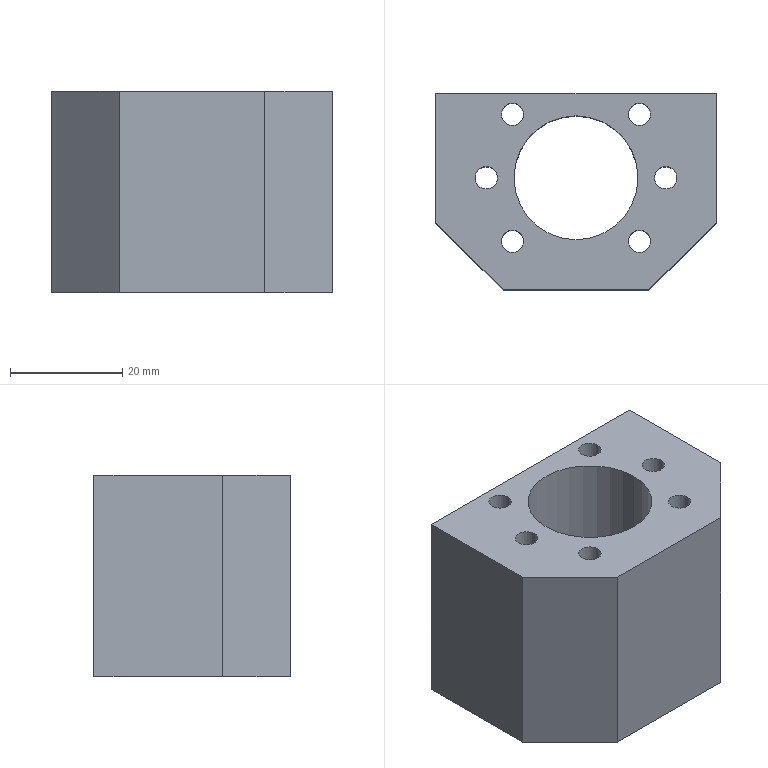Part | SolidWorks | features BaseBody 1 | 1 solid | 34 faces | box 50 x 35 x 36 mm | volume 40507 mm3 | cylinder 22 | plane 12 | commonest cylinder face diameters 4 x12 5 x8 22.1 x2
STEP:
#1=CARTESIAN_POINT('',(-15.,5.,6.));
#2=VERTEX_POINT('',#1);
#3=CARTESIAN_POINT('',(-20.,5.,6.));
#4=VERTEX_POINT('',#3);
#5=CARTESIAN_POINT('',(-17.5,5.,6.));
#6=DIRECTION('',(0.,1.,0.));
#7=DIRECTION('',(-1.,0.,0.));
#8=AXIS2_PLACEMENT_3D('',#5,#6,#7);
#9=CIRCLE('',#8,2.5);
#10=EDGE_CURVE('',#2,#4,#9,.T.);
#11=ORIENTED_EDGE('',*,*,#10,.F.);
#12=CARTESIAN_POINT('',(-15.,15.,6.));
#13=VERTEX_POINT('',#12);
#14=CARTESIAN_POINT('',(-15.,5.,6.));
#15=DIRECTION('',(0.,1.,0.));
#16=VECTOR('',#15,1000.);
#17=LINE('',#14,#16);
#18=EDGE_CURVE('',#2,#13,#17,.T.);
#19=ORIENTED_EDGE('',*,*,#18,.T.);
#20=CARTESIAN_POINT('',(-20.,15.,6.));
#21=VERTEX_POINT('',#20);
#22=CARTESIAN_POINT('',(-17.5,15.,6.));
#23=DIRECTION('',(0.,1.,0.));
#24=DIRECTION('',(-1.,0.,0.));
#25=AXIS2_PLACEMENT_3D('',#22,#23,#24);
#26=CIRCLE('',#25,2.5);
#27=EDGE_CURVE('',#13,#21,#26,.T.);
#28=ORIENTED_EDGE('',*,*,#27,.T.);
#29=CARTESIAN_POINT('',(-20.,5.,6.));
#30=DIRECTION('',(0.,1.,0.));
#31=VECTOR('',#30,1000.);
#32=LINE('',#29,#31);
#33=EDGE_CURVE('',#4,#21,#32,.T.);
#34=ORIENTED_EDGE('',*,*,#33,.F.);
#35=EDGE_LOOP('',(#11,#19,#28,#34));
#36=FACE_OUTER_BOUND('',#35,.T.);
#37=CARTESIAN_POINT('',(-17.5,5.,6.));
#38=DIRECTION('',(0.,1.,0.));
#39=DIRECTION('',(-1.,0.,0.));
#40=AXIS2_PLACEMENT_3D('',#37,#38,#39);
#41=CYLINDRICAL_SURFACE('',#40,2.5);
#42=ADVANCED_FACE('',(#36),#41,.F.);
#43=CARTESIAN_POINT('',(-15.,5.,30.));
#44=VERTEX_POINT('',#43);
#45=CARTESIAN_POINT('',(-20.,5.,30.));
#46=VERTEX_POINT('',#45);
#47=CARTESIAN_POINT('',(-17.5,5.,30.));
#48=DIRECTION('',(0.,1.,0.));
#49=DIRECTION('',(-1.,0.,0.));
#50=AXIS2_PLACEMENT_3D('',#47,#48,#49);
#51=CIRCLE('',#50,2.5);
#52=EDGE_CURVE('',#44,#46,#51,.T.);
#53=ORIENTED_EDGE('',*,*,#52,.F.);
#54=CARTESIAN_POINT('',(-15.,15.,30.));
#55=VERTEX_POINT('',#54);
#56=CARTESIAN_POINT('',(-15.,5.,30.));
#57=DIRECTION('',(0.,1.,0.));
#58=VECTOR('',#57,1000.);
#59=LINE('',#56,#58);
#60=EDGE_CURVE('',#44,#55,#59,.T.);
#61=ORIENTED_EDGE('',*,*,#60,.T.);
#62=CARTESIAN_POINT('',(-20.,15.,30.));
#63=VERTEX_POINT('',#62);
#64=CARTESIAN_POINT('',(-17.5,15.,30.));
#65=DIRECTION('',(0.,1.,0.));
#66=DIRECTION('',(-1.,0.,0.));
#67=AXIS2_PLACEMENT_3D('',#64,#65,#66);
#68=CIRCLE('',#67,2.5);
#69=EDGE_CURVE('',#55,#63,#68,.T.);
#70=ORIENTED_EDGE('',*,*,#69,.T.);
#71=CARTESIAN_POINT('',(-20.,5.,30.));
#72=DIRECTION('',(0.,1.,0.));
#73=VECTOR('',#72,1000.);
#74=LINE('',#71,#73);
#75=EDGE_CURVE('',#46,#63,#74,.T.);
#76=ORIENTED_EDGE('',*,*,#75,.F.);
#77=EDGE_LOOP('',(#53,#61,#70,#76));
#78=FACE_OUTER_BOUND('',#77,.T.);
#79=CARTESIAN_POINT('',(-17.5,5.,30.));
#80=DIRECTION('',(0.,1.,0.));
#81=DIRECTION('',(-1.,0.,0.));
#82=AXIS2_PLACEMENT_3D('',#79,#80,#81);
#83=CYLINDRICAL_SURFACE('',#82,2.5);
#84=ADVANCED_FACE('',(#78),#83,.F.);
#85=CARTESIAN_POINT('',(20.,5.,30.));
#86=VERTEX_POINT('',#85);
#87=CARTESIAN_POINT('',(15.,5.,30.));
#88=VERTEX_POINT('',#87);
#89=CARTESIAN_POINT('',(17.5,5.,30.));
#90=DIRECTION('',(0.,1.,0.));
#91=DIRECTION('',(-1.,0.,0.));
#92=AXIS2_PLACEMENT_3D('',#89,#90,#91);
#93=CIRCLE('',#92,2.5);
#94=EDGE_CURVE('',#86,#88,#93,.T.);
#95=ORIENTED_EDGE('',*,*,#94,.F.);
#96=CARTESIAN_POINT('',(20.,15.,30.));
#97=VERTEX_POINT('',#96);
#98=CARTESIAN_POINT('',(20.,5.,30.));
#99=DIRECTION('',(0.,1.,0.));
#100=VECTOR('',#99,1000.);
#101=LINE('',#98,#100);
#102=EDGE_CURVE('',#86,#97,#101,.T.);
#103=ORIENTED_EDGE('',*,*,#102,.T.);
#104=CARTESIAN_POINT('',(15.,15.,30.));
#105=VERTEX_POINT('',#104);
#106=CARTESIAN_POINT('',(17.5,15.,30.));
#107=DIRECTION('',(0.,1.,0.));
#108=DIRECTION('',(-1.,0.,0.));
#109=AXIS2_PLACEMENT_3D('',#106,#107,#108);
#110=CIRCLE('',#109,2.5);
#111=EDGE_CURVE('',#97,#105,#110,.T.);
#112=ORIENTED_EDGE('',*,*,#111,.T.);
#113=CARTESIAN_POINT('',(15.,5.,30.));
#114=DIRECTION('',(0.,1.,0.));
#115=VECTOR('',#114,1000.);
#116=LINE('',#113,#115);
#117=EDGE_CURVE('',#88,#105,#116,.T.);
#118=ORIENTED_EDGE('',*,*,#117,.F.);
#119=EDGE_LOOP('',(#95,#103,#112,#118));
#120=FACE_OUTER_BOUND('',#119,.T.);
#121=CARTESIAN_POINT('',(17.5,5.,30.));
#122=DIRECTION('',(0.,1.,0.));
#123=DIRECTION('',(-1.,0.,0.));
#124=AXIS2_PLACEMENT_3D('',#121,#122,#123);
#125=CYLINDRICAL_SURFACE('',#124,2.5);
#126=ADVANCED_FACE('',(#120),#125,.F.);
#127=CARTESIAN_POINT('',(20.,5.,6.));
#128=VERTEX_POINT('',#127);
#129=CARTESIAN_POINT('',(15.,5.,6.));
#130=VERTEX_POINT('',#129);
#131=CARTESIAN_POINT('',(17.5,5.,6.));
#132=DIRECTION('',(0.,1.,0.));
#133=DIRECTION('',(-1.,0.,0.));
#134=AXIS2_PLACEMENT_3D('',#131,#132,#133);
#135=CIRCLE('',#134,2.5);
#136=EDGE_CURVE('',#128,#130,#135,.T.);
#137=ORIENTED_EDGE('',*,*,#136,.F.);
#138=CARTESIAN_POINT('',(20.,15.,6.));
#139=VERTEX_POINT('',#138);
#140=CARTESIAN_POINT('',(20.,5.,6.));
#141=DIRECTION('',(0.,1.,0.));
#142=VECTOR('',#141,1000.);
#143=LINE('',#140,#142);
#144=EDGE_CURVE('',#128,#139,#143,.T.);
#145=ORIENTED_EDGE('',*,*,#144,.T.);
#146=CARTESIAN_POINT('',(15.,15.,6.));
#147=VERTEX_POINT('',#146);
#148=CARTESIAN_POINT('',(17.5,15.,6.));
#149=DIRECTION('',(0.,1.,0.));
#150=DIRECTION('',(-1.,0.,0.));
#151=AXIS2_PLACEMENT_3D('',#148,#149,#150);
#152=CIRCLE('',#151,2.5);
#153=EDGE_CURVE('',#139,#147,#152,.T.);
#154=ORIENTED_EDGE('',*,*,#153,.T.);
#155=CARTESIAN_POINT('',(15.,5.,6.));
#156=DIRECTION('',(0.,1.,0.));
#157=VECTOR('',#156,1000.);
#158=LINE('',#155,#157);
#159=EDGE_CURVE('',#130,#147,#158,.T.);
#160=ORIENTED_EDGE('',*,*,#159,.F.);
#161=EDGE_LOOP('',(#137,#145,#154,#160));
#162=FACE_OUTER_BOUND('',#161,.T.);
#163=CARTESIAN_POINT('',(17.5,5.,6.));
#164=DIRECTION('',(0.,1.,0.));
#165=DIRECTION('',(-1.,0.,0.));
#166=AXIS2_PLACEMENT_3D('',#163,#164,#165);
#167=CYLINDRICAL_SURFACE('',#166,2.5);
#168=ADVANCED_FACE('',(#162),#167,.F.);
#169=CARTESIAN_POINT('',(18.,0.,36.));
#170=VERTEX_POINT('',#169);
#171=CARTESIAN_POINT('',(14.,0.,36.));
#172=VERTEX_POINT('',#171);
#173=CARTESIAN_POINT('',(16.,0.,36.));
#174=DIRECTION('',(0.,0.,-1.));
#175=DIRECTION('',(-1.,0.,0.));
#176=AXIS2_PLACEMENT_3D('',#173,#174,#175);
#177=CIRCLE('',#176,2.);
#178=EDGE_CURVE('',#170,#172,#177,.T.);
#179=ORIENTED_EDGE('',*,*,#178,.F.);
#180=CARTESIAN_POINT('',(18.,0.,0.));
#181=VERTEX_POINT('',#180);
#182=CARTESIAN_POINT('',(18.,0.,36.));
#183=DIRECTION('',(0.,0.,-1.));
#184=VECTOR('',#183,1000.);
#185=LINE('',#182,#184);
#186=EDGE_CURVE('',#170,#181,#185,.T.);
#187=ORIENTED_EDGE('',*,*,#186,.T.);
#188=CARTESIAN_POINT('',(14.,0.,0.));
#189=VERTEX_POINT('',#188);
#190=CARTESIAN_POINT('',(16.,0.,0.));
#191=DIRECTION('',(0.,0.,-1.));
#192=DIRECTION('',(-1.,0.,0.));
#193=AXIS2_PLACEMENT_3D('',#190,#191,#192);
#194=CIRCLE('',#193,2.);
#195=EDGE_CURVE('',#181,#189,#194,.T.);
#196=ORIENTED_EDGE('',*,*,#195,.T.);
#197=CARTESIAN_POINT('',(14.,0.,36.));
#198=DIRECTION('',(0.,0.,-1.));
#199=VECTOR('',#198,1000.);
#200=LINE('',#197,#199);
#201=EDGE_CURVE('',#172,#189,#200,.T.);
#202=ORIENTED_EDGE('',*,*,#201,.F.);
#203=EDGE_LOOP('',(#179,#187,#196,#202));
#204=FACE_OUTER_BOUND('',#203,.T.);
#205=CARTESIAN_POINT('',(16.,0.,36.));
#206=DIRECTION('',(0.,0.,-1.));
#207=DIRECTION('',(-1.,0.,0.));
#208=AXIS2_PLACEMENT_3D('',#205,#206,#207);
#209=CYLINDRICAL_SURFACE('',#208,2.);
#210=ADVANCED_FACE('',(#204),#209,.F.);
#211=CARTESIAN_POINT('',(13.314,11.314,36.));
#212=VERTEX_POINT('',#211);
#213=CARTESIAN_POINT('',(9.314,11.314,36.));
#214=VERTEX_POINT('',#213);
#215=CARTESIAN_POINT('',(11.314,11.314,36.));
#216=DIRECTION('',(0.,0.,-1.));
#217=DIRECTION('',(-1.,0.,0.));
#218=AXIS2_PLACEMENT_3D('',#215,#216,#217);
#219=CIRCLE('',#218,2.);
#220=EDGE_CURVE('',#212,#214,#219,.T.);
#221=ORIENTED_EDGE('',*,*,#220,.F.);
#222=CARTESIAN_POINT('',(13.314,11.314,0.));
#223=VERTEX_POINT('',#222);
#224=CARTESIAN_POINT('',(13.314,11.314,36.));
#225=DIRECTION('',(0.,0.,-1.));
#226=VECTOR('',#225,1000.);
#227=LINE('',#224,#226);
#228=EDGE_CURVE('',#212,#223,#227,.T.);
#229=ORIENTED_EDGE('',*,*,#228,.T.);
#230=CARTESIAN_POINT('',(9.314,11.314,0.));
#231=VERTEX_POINT('',#230);
#232=CARTESIAN_POINT('',(11.314,11.314,0.));
#233=DIRECTION('',(0.,0.,-1.));
#234=DIRECTION('',(-1.,0.,0.));
#235=AXIS2_PLACEMENT_3D('',#232,#233,#234);
#236=CIRCLE('',#235,2.);
#237=EDGE_CURVE('',#223,#231,#236,.T.);
#238=ORIENTED_EDGE('',*,*,#237,.T.);
#239=CARTESIAN_POINT('',(9.314,11.314,36.));
#240=DIRECTION('',(0.,0.,-1.));
#241=VECTOR('',#240,1000.);
#242=LINE('',#239,#241);
#243=EDGE_CURVE('',#214,#231,#242,.T.);
#244=ORIENTED_EDGE('',*,*,#243,.F.);
#245=EDGE_LOOP('',(#221,#229,#238,#244));
#246=FACE_OUTER_BOUND('',#245,.T.);
#247=CARTESIAN_POINT('',(11.314,11.314,36.));
#248=DIRECTION('',(0.,0.,-1.));
#249=DIRECTION('',(-1.,0.,0.));
#250=AXIS2_PLACEMENT_3D('',#247,#248,#249);
#251=CYLINDRICAL_SURFACE('',#250,2.);
#252=ADVANCED_FACE('',(#246),#251,.F.);
#253=CARTESIAN_POINT('',(13.314,-11.314,36.));
#254=VERTEX_POINT('',#253);
#255=CARTESIAN_POINT('',(9.314,-11.314,36.));
#256=VERTEX_POINT('',#255);
#257=CARTESIAN_POINT('',(11.314,-11.314,36.));
#258=DIRECTION('',(0.,0.,-1.));
#259=DIRECTION('',(-1.,0.,0.));
#260=AXIS2_PLACEMENT_3D('',#257,#258,#259);
#261=CIRCLE('',#260,2.);
#262=EDGE_CURVE('',#254,#256,#261,.T.);
#263=ORIENTED_EDGE('',*,*,#262,.F.);
#264=CARTESIAN_POINT('',(13.314,-11.314,0.));
#265=VERTEX_POINT('',#264);
#266=CARTESIAN_POINT('',(13.314,-11.314,36.));
#267=DIRECTION('',(0.,0.,-1.));
#268=VECTOR('',#267,1000.);
#269=LINE('',#266,#268);
#270=EDGE_CURVE('',#254,#265,#269,.T.);
#271=ORIENTED_EDGE('',*,*,#270,.T.);
#272=CARTESIAN_POINT('',(9.314,-11.314,0.));
#273=VERTEX_POINT('',#272);
#274=CARTESIAN_POINT('',(11.314,-11.314,0.));
#275=DIRECTION('',(0.,0.,-1.));
#276=DIRECTION('',(-1.,0.,0.));
#277=AXIS2_PLACEMENT_3D('',#274,#275,#276);
#278=CIRCLE('',#277,2.);
#279=EDGE_CURVE('',#265,#273,#278,.T.);
#280=ORIENTED_EDGE('',*,*,#279,.T.);
#281=CARTESIAN_POINT('',(9.314,-11.314,36.));
#282=DIRECTION('',(0.,0.,-1.));
#283=VECTOR('',#282,1000.);
#284=LINE('',#281,#283);
#285=EDGE_CURVE('',#256,#273,#284,.T.);
#286=ORIENTED_EDGE('',*,*,#285,.F.);
#287=EDGE_LOOP('',(#263,#271,#280,#286));
#288=FACE_OUTER_BOUND('',#287,.T.);
#289=CARTESIAN_POINT('',(11.314,-11.314,36.));
#290=DIRECTION('',(0.,0.,-1.));
#291=DIRECTION('',(-1.,0.,0.));
#292=AXIS2_PLACEMENT_3D('',#289,#290,#291);
#293=CYLINDRICAL_SURFACE('',#292,2.);
#294=ADVANCED_FACE('',(#288),#293,.F.);
#295=CARTESIAN_POINT('',(-9.314,-11.314,36.));
#296=VERTEX_POINT('',#295);
#297=CARTESIAN_POINT('',(-13.314,-11.314,36.));
#298=VERTEX_POINT('',#297);
#299=CARTESIAN_POINT('',(-11.314,-11.314,36.));
#300=DIRECTION('',(0.,0.,-1.));
#301=DIRECTION('',(-1.,0.,0.));
#302=AXIS2_PLACEMENT_3D('',#299,#300,#301);
#303=CIRCLE('',#302,2.);
#304=EDGE_CURVE('',#296,#298,#303,.T.);
#305=ORIENTED_EDGE('',*,*,#304,.F.);
#306=CARTESIAN_POINT('',(-9.314,-11.314,0.));
#307=VERTEX_POINT('',#306);
#308=CARTESIAN_POINT('',(-9.314,-11.314,36.));
#309=DIRECTION('',(0.,0.,-1.));
#310=VECTOR('',#309,1000.);
#311=LINE('',#308,#310);
#312=EDGE_CURVE('',#296,#307,#311,.T.);
#313=ORIENTED_EDGE('',*,*,#312,.T.);
#314=CARTESIAN_POINT('',(-13.314,-11.314,0.));
#315=VERTEX_POINT('',#314);
#316=CARTESIAN_POINT('',(-11.314,-11.314,0.));
#317=DIRECTION('',(0.,0.,-1.));
#318=DIRECTION('',(-1.,0.,0.));
#319=AXIS2_PLACEMENT_3D('',#316,#317,#318);
#320=CIRCLE('',#319,2.);
#321=EDGE_CURVE('',#307,#315,#320,.T.);
#322=ORIENTED_EDGE('',*,*,#321,.T.);
#323=CARTESIAN_POINT('',(-13.314,-11.314,36.));
#324=DIRECTION('',(0.,0.,-1.));
#325=VECTOR('',#324,1000.);
#326=LINE('',#323,#325);
#327=EDGE_CURVE('',#298,#315,#326,.T.);
#328=ORIENTED_EDGE('',*,*,#327,.F.);
#329=EDGE_LOOP('',(#305,#313,#322,#328));
#330=FACE_OUTER_BOUND('',#329,.T.);
#331=CARTESIAN_POINT('',(-11.314,-11.314,36.));
#332=DIRECTION('',(0.,0.,-1.));
#333=DIRECTION('',(-1.,0.,0.));
#334=AXIS2_PLACEMENT_3D('',#331,#332,#333);
#335=CYLINDRICAL_SURFACE('',#334,2.);
#336=ADVANCED_FACE('',(#330),#335,.F.);
#337=CARTESIAN_POINT('',(-9.314,11.314,36.));
#338=VERTEX_POINT('',#337);
#339=CARTESIAN_POINT('',(-13.314,11.314,36.));
#340=VERTEX_POINT('',#339);
#341=CARTESIAN_POINT('',(-11.314,11.314,36.));
#342=DIRECTION('',(0.,0.,-1.));
#343=DIRECTION('',(-1.,0.,0.));
#344=AXIS2_PLACEMENT_3D('',#341,#342,#343);
#345=CIRCLE('',#344,2.);
#346=EDGE_CURVE('',#338,#340,#345,.T.);
#347=ORIENTED_EDGE('',*,*,#346,.F.);
#348=CARTESIAN_POINT('',(-9.314,11.314,0.));
#349=VERTEX_POINT('',#348);
#350=CARTESIAN_POINT('',(-9.314,11.314,36.));
#351=DIRECTION('',(0.,0.,-1.));
#352=VECTOR('',#351,1000.);
#353=LINE('',#350,#352);
#354=EDGE_CURVE('',#338,#349,#353,.T.);
#355=ORIENTED_EDGE('',*,*,#354,.T.);
#356=CARTESIAN_POINT('',(-13.314,11.314,0.));
#357=VERTEX_POINT('',#356);
#358=CARTESIAN_POINT('',(-11.314,11.314,0.));
#359=DIRECTION('',(0.,0.,-1.));
#360=DIRECTION('',(-1.,0.,0.));
#361=AXIS2_PLACEMENT_3D('',#358,#359,#360);
#362=CIRCLE('',#361,2.);
#363=EDGE_CURVE('',#349,#357,#362,.T.);
#364=ORIENTED_EDGE('',*,*,#363,.T.);
#365=CARTESIAN_POINT('',(-13.314,11.314,36.));
#366=DIRECTION('',(0.,0.,-1.));
#367=VECTOR('',#366,1000.);
#368=LINE('',#365,#367);
#369=EDGE_CURVE('',#340,#357,#368,.T.);
#370=ORIENTED_EDGE('',*,*,#369,.F.);
#371=EDGE_LOOP('',(#347,#355,#364,#370));
#372=FACE_OUTER_BOUND('',#371,.T.);
#373=CARTESIAN_POINT('',(-11.314,11.314,36.));
#374=DIRECTION('',(0.,0.,-1.));
#375=DIRECTION('',(-1.,0.,0.));
#376=AXIS2_PLACEMENT_3D('',#373,#374,#375);
#377=CYLINDRICAL_SURFACE('',#376,2.);
#378=ADVANCED_FACE('',(#372),#377,.F.);
#379=CARTESIAN_POINT('',(-14.,0.,36.));
#380=VERTEX_POINT('',#379);
#381=CARTESIAN_POINT('',(-18.,0.,36.));
#382=VERTEX_POINT('',#381);
#383=CARTESIAN_POINT('',(-16.,0.,36.));
#384=DIRECTION('',(0.,0.,-1.));
#385=DIRECTION('',(-1.,0.,0.));
#386=AXIS2_PLACEMENT_3D('',#383,#384,#385);
#387=CIRCLE('',#386,2.);
#388=EDGE_CURVE('',#380,#382,#387,.T.);
#389=ORIENTED_EDGE('',*,*,#388,.F.);
#390=CARTESIAN_POINT('',(-14.,0.,0.));
#391=VERTEX_POINT('',#390);
#392=CARTESIAN_POINT('',(-14.,0.,36.));
#393=DIRECTION('',(0.,0.,-1.));
#394=VECTOR('',#393,1000.);
#395=LINE('',#392,#394);
#396=EDGE_CURVE('',#380,#391,#395,.T.);
#397=ORIENTED_EDGE('',*,*,#396,.T.);
#398=CARTESIAN_POINT('',(-18.,0.,0.));
#399=VERTEX_POINT('',#398);
#400=CARTESIAN_POINT('',(-16.,0.,0.));
#401=DIRECTION('',(0.,0.,-1.));
#402=DIRECTION('',(-1.,0.,0.));
#403=AXIS2_PLACEMENT_3D('',#400,#401,#402);
#404=CIRCLE('',#403,2.);
#405=EDGE_CURVE('',#391,#399,#404,.T.);
#406=ORIENTED_EDGE('',*,*,#405,.T.);
#407=CARTESIAN_POINT('',(-18.,0.,36.));
#408=DIRECTION('',(0.,0.,-1.));
#409=VECTOR('',#408,1000.);
#410=LINE('',#407,#409);
#411=EDGE_CURVE('',#382,#399,#410,.T.);
#412=ORIENTED_EDGE('',*,*,#411,.F.);
#413=EDGE_LOOP('',(#389,#397,#406,#412));
#414=FACE_OUTER_BOUND('',#413,.T.);
#415=CARTESIAN_POINT('',(-16.,0.,36.));
#416=DIRECTION('',(0.,0.,-1.));
#417=DIRECTION('',(-1.,0.,0.));
#418=AXIS2_PLACEMENT_3D('',#415,#416,#417);
#419=CYLINDRICAL_SURFACE('',#418,2.);
#420=ADVANCED_FACE('',(#414),#419,.F.);
#421=CARTESIAN_POINT('',(11.05,0.,36.));
#422=VERTEX_POINT('',#421);
#423=CARTESIAN_POINT('',(-11.05,0.,36.));
#424=VERTEX_POINT('',#423);
#425=CARTESIAN_POINT('',(0.,0.,36.));
#426=DIRECTION('',(0.,0.,-1.));
#427=DIRECTION('',(-1.,0.,0.));
#428=AXIS2_PLACEMENT_3D('',#425,#426,#427);
#429=CIRCLE('',#428,11.05);
#430=EDGE_CURVE('',#422,#424,#429,.T.);
#431=ORIENTED_EDGE('',*,*,#430,.F.);
#432=CARTESIAN_POINT('',(11.05,0.,0.));
#433=VERTEX_POINT('',#432);
#434=CARTESIAN_POINT('',(11.05,0.,36.));
#435=DIRECTION('',(0.,0.,-1.));
#436=VECTOR('',#435,1000.);
#437=LINE('',#434,#436);
#438=EDGE_CURVE('',#422,#433,#437,.T.);
#439=ORIENTED_EDGE('',*,*,#438,.T.);
#440=CARTESIAN_POINT('',(-11.05,0.,0.));
#441=VERTEX_POINT('',#440);
#442=CARTESIAN_POINT('',(0.,0.,0.));
#443=DIRECTION('',(0.,0.,-1.));
#444=DIRECTION('',(-1.,0.,0.));
#445=AXIS2_PLACEMENT_3D('',#442,#443,#444);
#446=CIRCLE('',#445,11.05);
#447=EDGE_CURVE('',#433,#441,#446,.T.);
#448=ORIENTED_EDGE('',*,*,#447,.T.);
#449=CARTESIAN_POINT('',(-11.05,0.,36.));
#450=DIRECTION('',(0.,0.,-1.));
#451=VECTOR('',#450,1000.);
#452=LINE('',#449,#451);
#453=EDGE_CURVE('',#424,#441,#452,.T.);
#454=ORIENTED_EDGE('',*,*,#453,.F.);
#455=EDGE_LOOP('',(#431,#439,#448,#454));
#456=FACE_OUTER_BOUND('',#455,.T.);
#457=CARTESIAN_POINT('',(0.,0.,36.));
#458=DIRECTION('',(0.,0.,-1.));
#459=DIRECTION('',(-1.,0.,0.));
#460=AXIS2_PLACEMENT_3D('',#457,#458,#459);
#461=CYLINDRICAL_SURFACE('',#460,11.05);
#462=ADVANCED_FACE('',(#456),#461,.F.);
#463=CARTESIAN_POINT('',(-25.,15.,36.));
#464=VERTEX_POINT('',#463);
#465=CARTESIAN_POINT('',(-25.,15.,0.));
#466=VERTEX_POINT('',#465);
#467=CARTESIAN_POINT('',(-25.,15.,36.));
#468=DIRECTION('',(0.,0.,-1.));
#469=VECTOR('',#468,1000.);
#470=LINE('',#467,#469);
#471=EDGE_CURVE('',#464,#466,#470,.T.);
#472=ORIENTED_EDGE('',*,*,#471,.F.);
#473=CARTESIAN_POINT('',(25.,15.,36.));
#474=VERTEX_POINT('',#473);
#475=CARTESIAN_POINT('',(25.,15.,36.));
#476=DIRECTION('',(-1.,0.,0.));
#477=VECTOR('',#476,1000.);
#478=LINE('',#475,#477);
#479=EDGE_CURVE('',#474,#464,#478,.T.);
#480=ORIENTED_EDGE('',*,*,#479,.F.);
#481=CARTESIAN_POINT('',(25.,15.,0.));
#482=VERTEX_POINT('',#481);
#483=CARTESIAN_POINT('',(25.,15.,36.));
#484=DIRECTION('',(0.,0.,1.));
#485=VECTOR('',#484,1000.);
#486=LINE('',#483,#485);
#487=EDGE_CURVE('',#482,#474,#486,.T.);
#488=ORIENTED_EDGE('',*,*,#487,.F.);
#489=CARTESIAN_POINT('',(25.,15.,0.));
#490=DIRECTION('',(1.,0.,0.));
#491=VECTOR('',#490,1000.);
#492=LINE('',#489,#491);
#493=EDGE_CURVE('',#466,#482,#492,.T.);
#494=ORIENTED_EDGE('',*,*,#493,.F.);
#495=EDGE_LOOP('',(#472,#480,#488,#494));
#496=FACE_OUTER_BOUND('',#495,.T.);
#497=CARTESIAN_POINT('',(-17.5,15.,6.));
#498=DIRECTION('',(0.,1.,0.));
#499=DIRECTION('',(-1.,0.,0.));
#500=AXIS2_PLACEMENT_3D('',#497,#498,#499);
#501=CIRCLE('',#500,2.5);
#502=EDGE_CURVE('',#21,#13,#501,.T.);
#503=ORIENTED_EDGE('',*,*,#502,.F.);
#504=ORIENTED_EDGE('',*,*,#27,.F.);
#505=EDGE_LOOP('',(#503,#504));
#506=FACE_BOUND('',#505,.T.);
#507=CARTESIAN_POINT('',(-17.5,15.,30.));
#508=DIRECTION('',(0.,1.,0.));
#509=DIRECTION('',(-1.,0.,0.));
#510=AXIS2_PLACEMENT_3D('',#507,#508,#509);
#511=CIRCLE('',#510,2.5);
#512=EDGE_CURVE('',#63,#55,#511,.T.);
#513=ORIENTED_EDGE('',*,*,#512,.F.);
#514=ORIENTED_EDGE('',*,*,#69,.F.);
#515=EDGE_LOOP('',(#513,#514));
#516=FACE_BOUND('',#515,.T.);
#517=CARTESIAN_POINT('',(17.5,15.,30.));
#518=DIRECTION('',(0.,1.,0.));
#519=DIRECTION('',(-1.,0.,0.));
#520=AXIS2_PLACEMENT_3D('',#517,#518,#519);
#521=CIRCLE('',#520,2.5);
#522=EDGE_CURVE('',#105,#97,#521,.T.);
#523=ORIENTED_EDGE('',*,*,#522,.F.);
#524=ORIENTED_EDGE('',*,*,#111,.F.);
#525=EDGE_LOOP('',(#523,#524));
#526=FACE_BOUND('',#525,.T.);
#527=CARTESIAN_POINT('',(17.5,15.,6.));
#528=DIRECTION('',(0.,1.,0.));
#529=DIRECTION('',(-1.,0.,0.));
#530=AXIS2_PLACEMENT_3D('',#527,#528,#529);
#531=CIRCLE('',#530,2.5);
#532=EDGE_CURVE('',#147,#139,#531,.T.);
#533=ORIENTED_EDGE('',*,*,#532,.F.);
#534=ORIENTED_EDGE('',*,*,#153,.F.);
#535=EDGE_LOOP('',(#533,#534));
#536=FACE_BOUND('',#535,.T.);
#537=CARTESIAN_POINT('',(25.,15.,36.));
#538=DIRECTION('',(0.,-1.,0.));
#539=DIRECTION('',(1.,0.,0.));
#540=AXIS2_PLACEMENT_3D('',#537,#538,#539);
#541=PLANE('',#540);
#542=ADVANCED_FACE('',(#496,#506,#516,#526,#536),#541,.F.);
#543=CARTESIAN_POINT('',(16.,0.,0.));
#544=DIRECTION('',(0.,0.,-1.));
#545=DIRECTION('',(-1.,0.,0.));
#546=AXIS2_PLACEMENT_3D('',#543,#544,#545);
#547=CIRCLE('',#546,2.);
#548=EDGE_CURVE('',#189,#181,#547,.T.);
#549=ORIENTED_EDGE('',*,*,#548,.F.);
#550=ORIENTED_EDGE('',*,*,#195,.F.);
#551=EDGE_LOOP('',(#549,#550));
#552=FACE_BOUND('',#551,.T.);
#553=CARTESIAN_POINT('',(11.314,11.314,0.));
#554=DIRECTION('',(0.,0.,-1.));
#555=DIRECTION('',(-1.,0.,0.));
#556=AXIS2_PLACEMENT_3D('',#553,#554,#555);
#557=CIRCLE('',#556,2.);
#558=EDGE_CURVE('',#231,#223,#557,.T.);
#559=ORIENTED_EDGE('',*,*,#558,.F.);
#560=ORIENTED_EDGE('',*,*,#237,.F.);
#561=EDGE_LOOP('',(#559,#560));
#562=FACE_BOUND('',#561,.T.);
#563=CARTESIAN_POINT('',(11.314,-11.314,0.));
#564=DIRECTION('',(0.,0.,-1.));
#565=DIRECTION('',(-1.,0.,0.));
#566=AXIS2_PLACEMENT_3D('',#563,#564,#565);
#567=CIRCLE('',#566,2.);
#568=EDGE_CURVE('',#273,#265,#567,.T.);
#569=ORIENTED_EDGE('',*,*,#568,.F.);
#570=ORIENTED_EDGE('',*,*,#279,.F.);
#571=EDGE_LOOP('',(#569,#570));
#572=FACE_BOUND('',#571,.T.);
#573=CARTESIAN_POINT('',(-11.314,-11.314,0.));
#574=DIRECTION('',(0.,0.,-1.));
#575=DIRECTION('',(-1.,0.,0.));
#576=AXIS2_PLACEMENT_3D('',#573,#574,#575);
#577=CIRCLE('',#576,2.);
#578=EDGE_CURVE('',#315,#307,#577,.T.);
#579=ORIENTED_EDGE('',*,*,#578,.F.);
#580=ORIENTED_EDGE('',*,*,#321,.F.);
#581=EDGE_LOOP('',(#579,#580));
#582=FACE_BOUND('',#581,.T.);
#583=CARTESIAN_POINT('',(-11.314,11.314,0.));
#584=DIRECTION('',(0.,0.,-1.));
#585=DIRECTION('',(-1.,0.,0.));
#586=AXIS2_PLACEMENT_3D('',#583,#584,#585);
#587=CIRCLE('',#586,2.);
#588=EDGE_CURVE('',#357,#349,#587,.T.);
#589=ORIENTED_EDGE('',*,*,#588,.F.);
#590=ORIENTED_EDGE('',*,*,#363,.F.);
#591=EDGE_LOOP('',(#589,#590));
#592=FACE_BOUND('',#591,.T.);
#593=CARTESIAN_POINT('',(-16.,0.,0.));
#594=DIRECTION('',(0.,0.,-1.));
#595=DIRECTION('',(-1.,0.,0.));
#596=AXIS2_PLACEMENT_3D('',#593,#594,#595);
#597=CIRCLE('',#596,2.);
#598=EDGE_CURVE('',#399,#391,#597,.T.);
#599=ORIENTED_EDGE('',*,*,#598,.F.);
#600=ORIENTED_EDGE('',*,*,#405,.F.);
#601=EDGE_LOOP('',(#599,#600));
#602=FACE_BOUND('',#601,.T.);
#603=CARTESIAN_POINT('',(0.,0.,0.));
#604=DIRECTION('',(0.,0.,-1.));
#605=DIRECTION('',(-1.,0.,0.));
#606=AXIS2_PLACEMENT_3D('',#603,#604,#605);
#607=CIRCLE('',#606,11.05);
#608=EDGE_CURVE('',#441,#433,#607,.T.);
#609=ORIENTED_EDGE('',*,*,#608,.F.);
#610=ORIENTED_EDGE('',*,*,#447,.F.);
#611=EDGE_LOOP('',(#609,#610));
#612=FACE_BOUND('',#611,.T.);
#613=ORIENTED_EDGE('',*,*,#493,.T.);
#614=CARTESIAN_POINT('',(25.,-8.,0.));
#615=VERTEX_POINT('',#614);
#616=CARTESIAN_POINT('',(25.,0.,0.));
#617=DIRECTION('',(0.,1.,0.));
#618=VECTOR('',#617,1000.);
#619=LINE('',#616,#618);
#620=EDGE_CURVE('',#615,#482,#619,.T.);
#621=ORIENTED_EDGE('',*,*,#620,.F.);
#622=CARTESIAN_POINT('',(13.,-20.,0.));
#623=VERTEX_POINT('',#622);
#624=CARTESIAN_POINT('',(13.,-20.,0.));
#625=DIRECTION('',(0.7071,0.7071,0.));
#626=VECTOR('',#625,1000.);
#627=LINE('',#624,#626);
#628=EDGE_CURVE('',#623,#615,#627,.T.);
#629=ORIENTED_EDGE('',*,*,#628,.F.);
#630=CARTESIAN_POINT('',(-13.,-20.,0.));
#631=VERTEX_POINT('',#630);
#632=CARTESIAN_POINT('',(0.,-20.,0.));
#633=DIRECTION('',(1.,0.,0.));
#634=VECTOR('',#633,1000.);
#635=LINE('',#632,#634);
#636=EDGE_CURVE('',#631,#623,#635,.T.);
#637=ORIENTED_EDGE('',*,*,#636,.F.);
#638=CARTESIAN_POINT('',(-25.,-8.,0.));
#639=VERTEX_POINT('',#638);
#640=CARTESIAN_POINT('',(-25.,-8.,0.));
#641=DIRECTION('',(0.7071,-0.7071,0.));
#642=VECTOR('',#641,1000.);
#643=LINE('',#640,#642);
#644=EDGE_CURVE('',#639,#631,#643,.T.);
#645=ORIENTED_EDGE('',*,*,#644,.F.);
#646=CARTESIAN_POINT('',(-25.,0.,0.));
#647=DIRECTION('',(0.,-1.,0.));
#648=VECTOR('',#647,1000.);
#649=LINE('',#646,#648);
#650=EDGE_CURVE('',#466,#639,#649,.T.);
#651=ORIENTED_EDGE('',*,*,#650,.F.);
#652=EDGE_LOOP('',(#613,#621,#629,#637,#645,#651));
#653=FACE_OUTER_BOUND('',#652,.T.);
#654=CARTESIAN_POINT('',(0.,0.,0.));
#655=DIRECTION('',(0.,0.,1.));
#656=DIRECTION('',(1.,0.,0.));
#657=AXIS2_PLACEMENT_3D('',#654,#655,#656);
#658=PLANE('',#657);
#659=ADVANCED_FACE('',(#552,#562,#572,#582,#592,#602,#612,#653),#658,.F.);
#660=CARTESIAN_POINT('',(-25.,-8.,36.));
#661=VERTEX_POINT('',#660);
#662=CARTESIAN_POINT('',(-25.,-8.,36.));
#663=DIRECTION('',(0.,0.,-1.));
#664=VECTOR('',#663,1000.);
#665=LINE('',#662,#664);
#666=EDGE_CURVE('',#661,#639,#665,.T.);
#667=ORIENTED_EDGE('',*,*,#666,.F.);
#668=CARTESIAN_POINT('',(-25.,15.,36.));
#669=DIRECTION('',(0.,-1.,0.));
#670=VECTOR('',#669,1000.);
#671=LINE('',#668,#670);
#672=EDGE_CURVE('',#464,#661,#671,.T.);
#673=ORIENTED_EDGE('',*,*,#672,.F.);
#674=ORIENTED_EDGE('',*,*,#471,.T.);
#675=ORIENTED_EDGE('',*,*,#650,.T.);
#676=EDGE_LOOP('',(#667,#673,#674,#675));
#677=FACE_OUTER_BOUND('',#676,.T.);
#678=CARTESIAN_POINT('',(-25.,15.,36.));
#679=DIRECTION('',(1.,0.,0.));
#680=DIRECTION('',(0.,1.,0.));
#681=AXIS2_PLACEMENT_3D('',#678,#679,#680);
#682=PLANE('',#681);
#683=ADVANCED_FACE('',(#677),#682,.F.);
#684=CARTESIAN_POINT('',(16.,0.,36.));
#685=DIRECTION('',(0.,0.,-1.));
#686=DIRECTION('',(-1.,0.,0.));
#687=AXIS2_PLACEMENT_3D('',#684,#685,#686);
#688=CIRCLE('',#687,2.);
#689=EDGE_CURVE('',#172,#170,#688,.T.);
#690=ORIENTED_EDGE('',*,*,#689,.T.);
#691=ORIENTED_EDGE('',*,*,#178,.T.);
#692=EDGE_LOOP('',(#690,#691));
#693=FACE_BOUND('',#692,.T.);
#694=CARTESIAN_POINT('',(11.314,-11.314,36.));
#695=DIRECTION('',(0.,0.,-1.));
#696=DIRECTION('',(-1.,0.,0.));
#697=AXIS2_PLACEMENT_3D('',#694,#695,#696);
#698=CIRCLE('',#697,2.);
#699=EDGE_CURVE('',#256,#254,#698,.T.);
#700=ORIENTED_EDGE('',*,*,#699,.T.);
#701=ORIENTED_EDGE('',*,*,#262,.T.);
#702=EDGE_LOOP('',(#700,#701));
#703=FACE_BOUND('',#702,.T.);
#704=CARTESIAN_POINT('',(-11.314,11.314,36.));
#705=DIRECTION('',(0.,0.,-1.));
#706=DIRECTION('',(-1.,0.,0.));
#707=AXIS2_PLACEMENT_3D('',#704,#705,#706);
#708=CIRCLE('',#707,2.);
#709=EDGE_CURVE('',#340,#338,#708,.T.);
#710=ORIENTED_EDGE('',*,*,#709,.T.);
#711=ORIENTED_EDGE('',*,*,#346,.T.);
#712=EDGE_LOOP('',(#710,#711));
#713=FACE_BOUND('',#712,.T.);
#714=CARTESIAN_POINT('',(0.,0.,36.));
#715=DIRECTION('',(0.,0.,-1.));
#716=DIRECTION('',(-1.,0.,0.));
#717=AXIS2_PLACEMENT_3D('',#714,#715,#716);
#718=CIRCLE('',#717,11.05);
#719=EDGE_CURVE('',#424,#422,#718,.T.);
#720=ORIENTED_EDGE('',*,*,#719,.T.);
#721=ORIENTED_EDGE('',*,*,#430,.T.);
#722=EDGE_LOOP('',(#720,#721));
#723=FACE_BOUND('',#722,.T.);
#724=CARTESIAN_POINT('',(25.,-8.,36.));
#725=VERTEX_POINT('',#724);
#726=CARTESIAN_POINT('',(25.,0.,36.));
#727=DIRECTION('',(0.,1.,0.));
#728=VECTOR('',#727,1000.);
#729=LINE('',#726,#728);
#730=EDGE_CURVE('',#725,#474,#729,.T.);
#731=ORIENTED_EDGE('',*,*,#730,.T.);
#732=ORIENTED_EDGE('',*,*,#479,.T.);
#733=ORIENTED_EDGE('',*,*,#672,.T.);
#734=CARTESIAN_POINT('',(-13.,-20.,36.));
#735=VERTEX_POINT('',#734);
#736=CARTESIAN_POINT('',(-25.,-8.,36.));
#737=DIRECTION('',(0.7071,-0.7071,0.));
#738=VECTOR('',#737,1000.);
#739=LINE('',#736,#738);
#740=EDGE_CURVE('',#661,#735,#739,.T.);
#741=ORIENTED_EDGE('',*,*,#740,.T.);
#742=CARTESIAN_POINT('',(13.,-20.,36.));
#743=VERTEX_POINT('',#742);
#744=CARTESIAN_POINT('',(0.,-20.,36.));
#745=DIRECTION('',(1.,0.,0.));
#746=VECTOR('',#745,1000.);
#747=LINE('',#744,#746);
#748=EDGE_CURVE('',#735,#743,#747,.T.);
#749=ORIENTED_EDGE('',*,*,#748,.T.);
#750=CARTESIAN_POINT('',(13.,-20.,36.));
#751=DIRECTION('',(0.7071,0.7071,0.));
#752=VECTOR('',#751,1000.);
#753=LINE('',#750,#752);
#754=EDGE_CURVE('',#743,#725,#753,.T.);
#755=ORIENTED_EDGE('',*,*,#754,.T.);
#756=EDGE_LOOP('',(#731,#732,#733,#741,#749,#755));
#757=FACE_OUTER_BOUND('',#756,.T.);
#758=CARTESIAN_POINT('',(-16.,0.,36.));
#759=DIRECTION('',(0.,0.,-1.));
#760=DIRECTION('',(-1.,0.,0.));
#761=AXIS2_PLACEMENT_3D('',#758,#759,#760);
#762=CIRCLE('',#761,2.);
#763=EDGE_CURVE('',#382,#380,#762,.T.);
#764=ORIENTED_EDGE('',*,*,#763,.T.);
#765=ORIENTED_EDGE('',*,*,#388,.T.);
#766=EDGE_LOOP('',(#764,#765));
#767=FACE_BOUND('',#766,.T.);
#768=CARTESIAN_POINT('',(-11.314,-11.314,36.));
#769=DIRECTION('',(0.,0.,-1.));
#770=DIRECTION('',(-1.,0.,0.));
#771=AXIS2_PLACEMENT_3D('',#768,#769,#770);
#772=CIRCLE('',#771,2.);
#773=EDGE_CURVE('',#298,#296,#772,.T.);
#774=ORIENTED_EDGE('',*,*,#773,.T.);
#775=ORIENTED_EDGE('',*,*,#304,.T.);
#776=EDGE_LOOP('',(#774,#775));
#777=FACE_BOUND('',#776,.T.);
#778=CARTESIAN_POINT('',(11.314,11.314,36.));
#779=DIRECTION('',(0.,0.,-1.));
#780=DIRECTION('',(-1.,0.,0.));
#781=AXIS2_PLACEMENT_3D('',#778,#779,#780);
#782=CIRCLE('',#781,2.);
#783=EDGE_CURVE('',#214,#212,#782,.T.);
#784=ORIENTED_EDGE('',*,*,#783,.T.);
#785=ORIENTED_EDGE('',*,*,#220,.T.);
#786=EDGE_LOOP('',(#784,#785));
#787=FACE_BOUND('',#786,.T.);
#788=CARTESIAN_POINT('',(0.,0.,36.));
#789=DIRECTION('',(0.,0.,1.));
#790=DIRECTION('',(1.,0.,0.));
#791=AXIS2_PLACEMENT_3D('',#788,#789,#790);
#792=PLANE('',#791);
#793=ADVANCED_FACE('',(#693,#703,#713,#723,#757,#767,#777,#787),#792,.T.);
#794=ORIENTED_EDGE('',*,*,#487,.T.);
#795=ORIENTED_EDGE('',*,*,#730,.F.);
#796=CARTESIAN_POINT('',(25.,-8.,36.));
#797=DIRECTION('',(0.,0.,1.));
#798=VECTOR('',#797,1000.);
#799=LINE('',#796,#798);
#800=EDGE_CURVE('',#615,#725,#799,.T.);
#801=ORIENTED_EDGE('',*,*,#800,.F.);
#802=ORIENTED_EDGE('',*,*,#620,.T.);
#803=EDGE_LOOP('',(#794,#795,#801,#802));
#804=FACE_OUTER_BOUND('',#803,.T.);
#805=CARTESIAN_POINT('',(25.,15.,36.));
#806=DIRECTION('',(-1.,0.,0.));
#807=DIRECTION('',(0.,-1.,0.));
#808=AXIS2_PLACEMENT_3D('',#805,#806,#807);
#809=PLANE('',#808);
#810=ADVANCED_FACE('',(#804),#809,.F.);
#811=ORIENTED_EDGE('',*,*,#18,.F.);
#812=CARTESIAN_POINT('',(-17.5,5.,6.));
#813=DIRECTION('',(0.,1.,0.));
#814=DIRECTION('',(-1.,0.,0.));
#815=AXIS2_PLACEMENT_3D('',#812,#813,#814);
#816=CIRCLE('',#815,2.5);
#817=EDGE_CURVE('',#4,#2,#816,.T.);
#818=ORIENTED_EDGE('',*,*,#817,.F.);
#819=ORIENTED_EDGE('',*,*,#33,.T.);
#820=ORIENTED_EDGE('',*,*,#502,.T.);
#821=EDGE_LOOP('',(#811,#818,#819,#820));
#822=FACE_OUTER_BOUND('',#821,.T.);
#823=CARTESIAN_POINT('',(-17.5,5.,6.));
#824=DIRECTION('',(0.,1.,0.));
#825=DIRECTION('',(-1.,0.,0.));
#826=AXIS2_PLACEMENT_3D('',#823,#824,#825);
#827=CYLINDRICAL_SURFACE('',#826,2.5);
#828=ADVANCED_FACE('',(#822),#827,.F.);
#829=ORIENTED_EDGE('',*,*,#60,.F.);
#830=CARTESIAN_POINT('',(-17.5,5.,30.));
#831=DIRECTION('',(0.,1.,0.));
#832=DIRECTION('',(-1.,0.,0.));
#833=AXIS2_PLACEMENT_3D('',#830,#831,#832);
#834=CIRCLE('',#833,2.5);
#835=EDGE_CURVE('',#46,#44,#834,.T.);
#836=ORIENTED_EDGE('',*,*,#835,.F.);
#837=ORIENTED_EDGE('',*,*,#75,.T.);
#838=ORIENTED_EDGE('',*,*,#512,.T.);
#839=EDGE_LOOP('',(#829,#836,#837,#838));
#840=FACE_OUTER_BOUND('',#839,.T.);
#841=CARTESIAN_POINT('',(-17.5,5.,30.));
#842=DIRECTION('',(0.,1.,0.));
#843=DIRECTION('',(-1.,0.,0.));
#844=AXIS2_PLACEMENT_3D('',#841,#842,#843);
#845=CYLINDRICAL_SURFACE('',#844,2.5);
#846=ADVANCED_FACE('',(#840),#845,.F.);
#847=ORIENTED_EDGE('',*,*,#102,.F.);
#848=CARTESIAN_POINT('',(17.5,5.,30.));
#849=DIRECTION('',(0.,1.,0.));
#850=DIRECTION('',(-1.,0.,0.));
#851=AXIS2_PLACEMENT_3D('',#848,#849,#850);
#852=CIRCLE('',#851,2.5);
#853=EDGE_CURVE('',#88,#86,#852,.T.);
#854=ORIENTED_EDGE('',*,*,#853,.F.);
#855=ORIENTED_EDGE('',*,*,#117,.T.);
#856=ORIENTED_EDGE('',*,*,#522,.T.);
#857=EDGE_LOOP('',(#847,#854,#855,#856));
#858=FACE_OUTER_BOUND('',#857,.T.);
#859=CARTESIAN_POINT('',(17.5,5.,30.));
#860=DIRECTION('',(0.,1.,0.));
#861=DIRECTION('',(-1.,0.,0.));
#862=AXIS2_PLACEMENT_3D('',#859,#860,#861);
#863=CYLINDRICAL_SURFACE('',#862,2.5);
#864=ADVANCED_FACE('',(#858),#863,.F.);
#865=ORIENTED_EDGE('',*,*,#144,.F.);
#866=CARTESIAN_POINT('',(17.5,5.,6.));
#867=DIRECTION('',(0.,1.,0.));
#868=DIRECTION('',(-1.,0.,0.));
#869=AXIS2_PLACEMENT_3D('',#866,#867,#868);
#870=CIRCLE('',#869,2.5);
#871=EDGE_CURVE('',#130,#128,#870,.T.);
#872=ORIENTED_EDGE('',*,*,#871,.F.);
#873=ORIENTED_EDGE('',*,*,#159,.T.);
#874=ORIENTED_EDGE('',*,*,#532,.T.);
#875=EDGE_LOOP('',(#865,#872,#873,#874));
#876=FACE_OUTER_BOUND('',#875,.T.);
#877=CARTESIAN_POINT('',(17.5,5.,6.));
#878=DIRECTION('',(0.,1.,0.));
#879=DIRECTION('',(-1.,0.,0.));
#880=AXIS2_PLACEMENT_3D('',#877,#878,#879);
#881=CYLINDRICAL_SURFACE('',#880,2.5);
#882=ADVANCED_FACE('',(#876),#881,.F.);
#883=ORIENTED_EDGE('',*,*,#186,.F.);
#884=ORIENTED_EDGE('',*,*,#689,.F.);
#885=ORIENTED_EDGE('',*,*,#201,.T.);
#886=ORIENTED_EDGE('',*,*,#548,.T.);
#887=EDGE_LOOP('',(#883,#884,#885,#886));
#888=FACE_OUTER_BOUND('',#887,.T.);
#889=CARTESIAN_POINT('',(16.,0.,36.));
#890=DIRECTION('',(0.,0.,-1.));
#891=DIRECTION('',(-1.,0.,0.));
#892=AXIS2_PLACEMENT_3D('',#889,#890,#891);
#893=CYLINDRICAL_SURFACE('',#892,2.);
#894=ADVANCED_FACE('',(#888),#893,.F.);
#895=ORIENTED_EDGE('',*,*,#228,.F.);
#896=ORIENTED_EDGE('',*,*,#783,.F.);
#897=ORIENTED_EDGE('',*,*,#243,.T.);
#898=ORIENTED_EDGE('',*,*,#558,.T.);
#899=EDGE_LOOP('',(#895,#896,#897,#898));
#900=FACE_OUTER_BOUND('',#899,.T.);
#901=CARTESIAN_POINT('',(11.314,11.314,36.));
#902=DIRECTION('',(0.,0.,-1.));
#903=DIRECTION('',(-1.,0.,0.));
#904=AXIS2_PLACEMENT_3D('',#901,#902,#903);
#905=CYLINDRICAL_SURFACE('',#904,2.);
#906=ADVANCED_FACE('',(#900),#905,.F.);
#907=ORIENTED_EDGE('',*,*,#270,.F.);
#908=ORIENTED_EDGE('',*,*,#699,.F.);
#909=ORIENTED_EDGE('',*,*,#285,.T.);
#910=ORIENTED_EDGE('',*,*,#568,.T.);
#911=EDGE_LOOP('',(#907,#908,#909,#910));
#912=FACE_OUTER_BOUND('',#911,.T.);
#913=CARTESIAN_POINT('',(11.314,-11.314,36.));
#914=DIRECTION('',(0.,0.,-1.));
#915=DIRECTION('',(-1.,0.,0.));
#916=AXIS2_PLACEMENT_3D('',#913,#914,#915);
#917=CYLINDRICAL_SURFACE('',#916,2.);
#918=ADVANCED_FACE('',(#912),#917,.F.);
#919=ORIENTED_EDGE('',*,*,#312,.F.);
#920=ORIENTED_EDGE('',*,*,#773,.F.);
#921=ORIENTED_EDGE('',*,*,#327,.T.);
#922=ORIENTED_EDGE('',*,*,#578,.T.);
#923=EDGE_LOOP('',(#919,#920,#921,#922));
#924=FACE_OUTER_BOUND('',#923,.T.);
#925=CARTESIAN_POINT('',(-11.314,-11.314,36.));
#926=DIRECTION('',(0.,0.,-1.));
#927=DIRECTION('',(-1.,0.,0.));
#928=AXIS2_PLACEMENT_3D('',#925,#926,#927);
#929=CYLINDRICAL_SURFACE('',#928,2.);
#930=ADVANCED_FACE('',(#924),#929,.F.);
#931=ORIENTED_EDGE('',*,*,#354,.F.);
#932=ORIENTED_EDGE('',*,*,#709,.F.);
#933=ORIENTED_EDGE('',*,*,#369,.T.);
#934=ORIENTED_EDGE('',*,*,#588,.T.);
#935=EDGE_LOOP('',(#931,#932,#933,#934));
#936=FACE_OUTER_BOUND('',#935,.T.);
#937=CARTESIAN_POINT('',(-11.314,11.314,36.));
#938=DIRECTION('',(0.,0.,-1.));
#939=DIRECTION('',(-1.,0.,0.));
#940=AXIS2_PLACEMENT_3D('',#937,#938,#939);
#941=CYLINDRICAL_SURFACE('',#940,2.);
#942=ADVANCED_FACE('',(#936),#941,.F.);
#943=ORIENTED_EDGE('',*,*,#396,.F.);
#944=ORIENTED_EDGE('',*,*,#763,.F.);
#945=ORIENTED_EDGE('',*,*,#411,.T.);
#946=ORIENTED_EDGE('',*,*,#598,.T.);
#947=EDGE_LOOP('',(#943,#944,#945,#946));
#948=FACE_OUTER_BOUND('',#947,.T.);
#949=CARTESIAN_POINT('',(-16.,0.,36.));
#950=DIRECTION('',(0.,0.,-1.));
#951=DIRECTION('',(-1.,0.,0.));
#952=AXIS2_PLACEMENT_3D('',#949,#950,#951);
#953=CYLINDRICAL_SURFACE('',#952,2.);
#954=ADVANCED_FACE('',(#948),#953,.F.);
#955=ORIENTED_EDGE('',*,*,#438,.F.);
#956=ORIENTED_EDGE('',*,*,#719,.F.);
#957=ORIENTED_EDGE('',*,*,#453,.T.);
#958=ORIENTED_EDGE('',*,*,#608,.T.);
#959=EDGE_LOOP('',(#955,#956,#957,#958));
#960=FACE_OUTER_BOUND('',#959,.T.);
#961=CARTESIAN_POINT('',(0.,0.,36.));
#962=DIRECTION('',(0.,0.,-1.));
#963=DIRECTION('',(-1.,0.,0.));
#964=AXIS2_PLACEMENT_3D('',#961,#962,#963);
#965=CYLINDRICAL_SURFACE('',#964,11.05);
#966=ADVANCED_FACE('',(#960),#965,.F.);
#967=ORIENTED_EDGE('',*,*,#800,.T.);
#968=ORIENTED_EDGE('',*,*,#754,.F.);
#969=CARTESIAN_POINT('',(13.,-20.,36.));
#970=DIRECTION('',(0.,0.,1.));
#971=VECTOR('',#970,1000.);
#972=LINE('',#969,#971);
#973=EDGE_CURVE('',#623,#743,#972,.T.);
#974=ORIENTED_EDGE('',*,*,#973,.F.);
#975=ORIENTED_EDGE('',*,*,#628,.T.);
#976=EDGE_LOOP('',(#967,#968,#974,#975));
#977=FACE_OUTER_BOUND('',#976,.T.);
#978=CARTESIAN_POINT('',(25.,-8.,36.));
#979=DIRECTION('',(-0.7071,0.7071,0.));
#980=DIRECTION('',(-0.7071,-0.7071,0.));
#981=AXIS2_PLACEMENT_3D('',#978,#979,#980);
#982=PLANE('',#981);
#983=ADVANCED_FACE('',(#977),#982,.F.);
#984=ORIENTED_EDGE('',*,*,#973,.T.);
#985=ORIENTED_EDGE('',*,*,#748,.F.);
#986=CARTESIAN_POINT('',(-13.,-20.,36.));
#987=DIRECTION('',(0.,0.,1.));
#988=VECTOR('',#987,1000.);
#989=LINE('',#986,#988);
#990=EDGE_CURVE('',#631,#735,#989,.T.);
#991=ORIENTED_EDGE('',*,*,#990,.F.);
#992=ORIENTED_EDGE('',*,*,#636,.T.);
#993=EDGE_LOOP('',(#984,#985,#991,#992));
#994=FACE_OUTER_BOUND('',#993,.T.);
#995=CARTESIAN_POINT('',(-13.,-20.,36.));
#996=DIRECTION('',(0.,1.,0.));
#997=DIRECTION('',(-1.,0.,0.));
#998=AXIS2_PLACEMENT_3D('',#995,#996,#997);
#999=PLANE('',#998);
#1000=ADVANCED_FACE('',(#994),#999,.F.);
#1001=ORIENTED_EDGE('',*,*,#990,.T.);
#1002=ORIENTED_EDGE('',*,*,#740,.F.);
#1003=ORIENTED_EDGE('',*,*,#666,.T.);
#1004=ORIENTED_EDGE('',*,*,#644,.T.);
#1005=EDGE_LOOP('',(#1001,#1002,#1003,#1004));
#1006=FACE_OUTER_BOUND('',#1005,.T.);
#1007=CARTESIAN_POINT('',(-25.,-8.,36.));
#1008=DIRECTION('',(0.7071,0.7071,0.));
#1009=DIRECTION('',(-0.7071,0.7071,0.));
#1010=AXIS2_PLACEMENT_3D('',#1007,#1008,#1009);
#1011=PLANE('',#1010);
#1012=ADVANCED_FACE('',(#1006),#1011,.F.);
#1013=ORIENTED_EDGE('',*,*,#817,.T.);
#1014=ORIENTED_EDGE('',*,*,#10,.T.);
#1015=EDGE_LOOP('',(#1013,#1014));
#1016=FACE_OUTER_BOUND('',#1015,.T.);
#1017=CARTESIAN_POINT('',(-17.5,5.,6.));
#1018=DIRECTION('',(0.,1.,0.));
#1019=DIRECTION('',(-1.,0.,0.));
#1020=AXIS2_PLACEMENT_3D('',#1017,#1018,#1019);
#1021=PLANE('',#1020);
#1022=ADVANCED_FACE('',(#1016),#1021,.T.);
#1023=ORIENTED_EDGE('',*,*,#835,.T.);
#1024=ORIENTED_EDGE('',*,*,#52,.T.);
#1025=EDGE_LOOP('',(#1023,#1024));
#1026=FACE_OUTER_BOUND('',#1025,.T.);
#1027=CARTESIAN_POINT('',(-17.5,5.,30.));
#1028=DIRECTION('',(0.,1.,0.));
#1029=DIRECTION('',(-1.,0.,0.));
#1030=AXIS2_PLACEMENT_3D('',#1027,#1028,#1029);
#1031=PLANE('',#1030);
#1032=ADVANCED_FACE('',(#1026),#1031,.T.);
#1033=ORIENTED_EDGE('',*,*,#853,.T.);
#1034=ORIENTED_EDGE('',*,*,#94,.T.);
#1035=EDGE_LOOP('',(#1033,#1034));
#1036=FACE_OUTER_BOUND('',#1035,.T.);
#1037=CARTESIAN_POINT('',(17.5,5.,30.));
#1038=DIRECTION('',(0.,-1.,0.));
#1039=DIRECTION('',(1.,0.,0.));
#1040=AXIS2_PLACEMENT_3D('',#1037,#1038,#1039);
#1041=PLANE('',#1040);
#1042=ADVANCED_FACE('',(#1036),#1041,.F.);
#1043=ORIENTED_EDGE('',*,*,#871,.T.);
#1044=ORIENTED_EDGE('',*,*,#136,.T.);
#1045=EDGE_LOOP('',(#1043,#1044));
#1046=FACE_OUTER_BOUND('',#1045,.T.);
#1047=CARTESIAN_POINT('',(17.5,5.,6.));
#1048=DIRECTION('',(0.,-1.,0.));
#1049=DIRECTION('',(1.,0.,0.));
#1050=AXIS2_PLACEMENT_3D('',#1047,#1048,#1049);
#1051=PLANE('',#1050);
#1052=ADVANCED_FACE('',(#1046),#1051,.F.);
#1053=CLOSED_SHELL('',(#42,#84,#126,#168,#210,#252,#294,#336,#378,#420,#462,#542,#659,#683,#793,#810,#828,#846,#864,#882,#894,#906,#918,#930,#942,#954,#966,#983,#1000,#1012,#1022,#1032,#1042,#1052));
#1054=MANIFOLD_SOLID_BREP('',#1053);
#1055=CARTESIAN_POINT('',(0.,0.,0.));
#1056=DIRECTION('',(0.,0.,1.));
#1057=DIRECTION('',(1.,0.,0.));
#1058=AXIS2_PLACEMENT_3D('',#1055,#1056,#1057);
#1059=(LENGTH_UNIT()NAMED_UNIT(*)SI_UNIT(.MILLI.,.METRE.));
#1060=UNCERTAINTY_MEASURE_WITH_UNIT(LENGTH_MEASURE(0.00001),#1059,'','');
#1061=(NAMED_UNIT(*)PLANE_ANGLE_UNIT()SI_UNIT($,.RADIAN.));
#1062=(NAMED_UNIT(*)SI_UNIT($,.STERADIAN.)SOLID_ANGLE_UNIT());
#1063=(GEOMETRIC_REPRESENTATION_CONTEXT(3)GLOBAL_UNCERTAINTY_ASSIGNED_CONTEXT((#1060))GLOBAL_UNIT_ASSIGNED_CONTEXT((#1059,#1061,#1062))REPRESENTATION_CONTEXT('',''));
#1064=ADVANCED_BREP_SHAPE_REPRESENTATION('',(#1054,#1058),#1063);